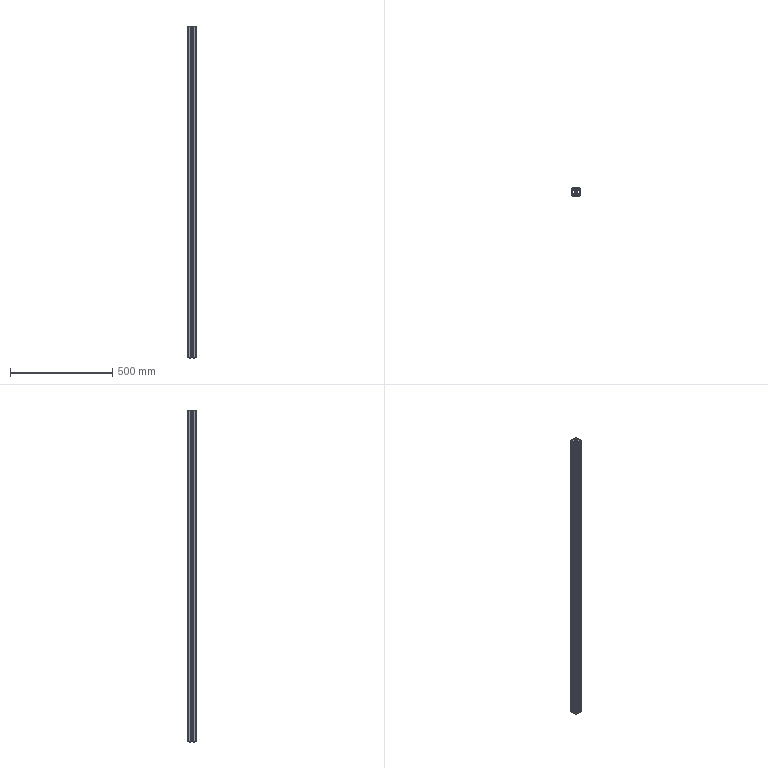Part | STEP file | LE-8-4040-S-OO_LE0311094953 | 1 solid | 248 faces | box 40 x 40 x 1620 mm | volume 773979 mm3 | cylinder 136 | plane 112 | commonest cylinder face diameters 0.6 x42 2 x28 4 x16 0.4 x14 6.6 x12 0.458 x8